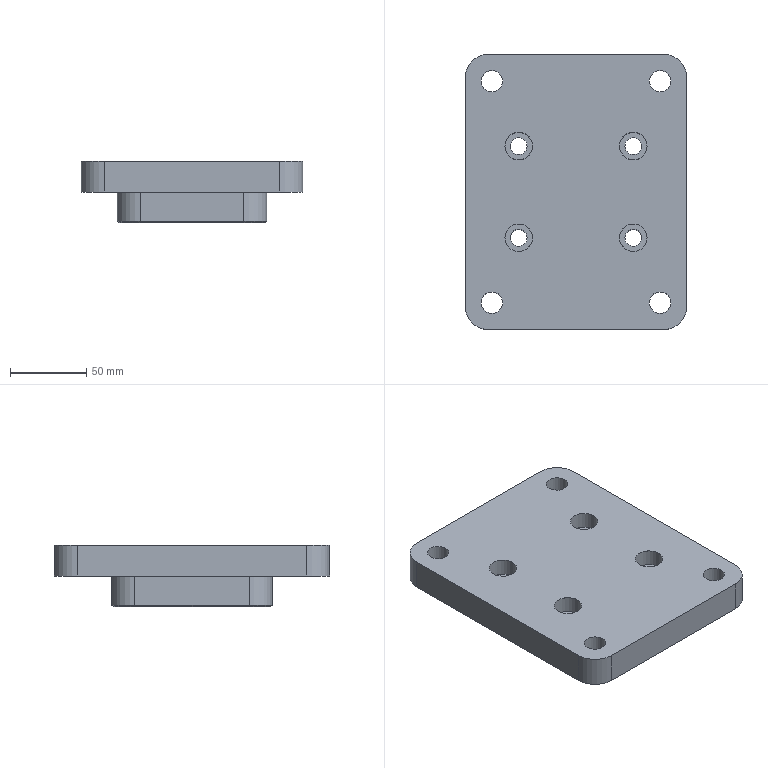Part | 1 solid | 47 faces | box 145 x 180 x 40 mm | volume 685350 mm3 | cylinder 20 | plane 19 | cone 8 | commonest cylinder face diameters 30 x8 11 x4 14 x4 18 x4
STEP:
#1=CARTESIAN_POINT('',(-32.,30.,-40.));
#2=VERTEX_POINT('',#1);
#3=CARTESIAN_POINT('',(-37.5,30.,-40.));
#4=DIRECTION('',(0.,0.,1.));
#5=DIRECTION('',(1.,0.,0.));
#6=AXIS2_PLACEMENT_3D('',#3,#4,#5);
#7=CIRCLE('',#6,5.5);
#8=EDGE_CURVE('',#2,#2,#7,.T.);
#9=ORIENTED_EDGE('',*,*,#8,.T.);
#10=EDGE_LOOP('',(#9));
#11=FACE_BOUND('',#10,.T.);
#12=CARTESIAN_POINT('',(43.,30.,-40.));
#13=VERTEX_POINT('',#12);
#14=CARTESIAN_POINT('',(37.5,30.,-40.));
#15=DIRECTION('',(0.,0.,1.));
#16=DIRECTION('',(1.,0.,0.));
#17=AXIS2_PLACEMENT_3D('',#14,#15,#16);
#18=CIRCLE('',#17,5.5);
#19=EDGE_CURVE('',#13,#13,#18,.T.);
#20=ORIENTED_EDGE('',*,*,#19,.T.);
#21=EDGE_LOOP('',(#20));
#22=FACE_BOUND('',#21,.T.);
#23=CARTESIAN_POINT('',(34.,51.5,-40.));
#24=VERTEX_POINT('',#23);
#25=CARTESIAN_POINT('',(48.,37.5,-40.));
#26=VERTEX_POINT('',#25);
#27=CARTESIAN_POINT('',(34.,37.5,-40.));
#28=DIRECTION('',(0.,0.,-1.));
#29=DIRECTION('',(-1.,0.,0.));
#30=AXIS2_PLACEMENT_3D('',#27,#28,#29);
#31=CIRCLE('',#30,14.);
#32=EDGE_CURVE('',#24,#26,#31,.T.);
#33=ORIENTED_EDGE('',*,*,#32,.T.);
#34=CARTESIAN_POINT('',(48.,-37.5,-40.));
#35=VERTEX_POINT('',#34);
#36=CARTESIAN_POINT('',(48.,-37.5,-40.));
#37=DIRECTION('',(0.,-1.,0.));
#38=VECTOR('',#37,1000.);
#39=LINE('',#36,#38);
#40=EDGE_CURVE('',#26,#35,#39,.T.);
#41=ORIENTED_EDGE('',*,*,#40,.T.);
#42=CARTESIAN_POINT('',(34.,-51.5,-40.));
#43=VERTEX_POINT('',#42);
#44=CARTESIAN_POINT('',(34.,-37.5,-40.));
#45=DIRECTION('',(0.,0.,-1.));
#46=DIRECTION('',(-1.,0.,0.));
#47=AXIS2_PLACEMENT_3D('',#44,#45,#46);
#48=CIRCLE('',#47,14.);
#49=EDGE_CURVE('',#35,#43,#48,.T.);
#50=ORIENTED_EDGE('',*,*,#49,.T.);
#51=CARTESIAN_POINT('',(-34.,-51.5,-40.));
#52=VERTEX_POINT('',#51);
#53=CARTESIAN_POINT('',(-34.,-51.5,-40.));
#54=DIRECTION('',(-1.,0.,0.));
#55=VECTOR('',#54,1000.);
#56=LINE('',#53,#55);
#57=EDGE_CURVE('',#43,#52,#56,.T.);
#58=ORIENTED_EDGE('',*,*,#57,.T.);
#59=CARTESIAN_POINT('',(-48.,-37.5,-40.));
#60=VERTEX_POINT('',#59);
#61=CARTESIAN_POINT('',(-34.,-37.5,-40.));
#62=DIRECTION('',(0.,0.,-1.));
#63=DIRECTION('',(-1.,0.,0.));
#64=AXIS2_PLACEMENT_3D('',#61,#62,#63);
#65=CIRCLE('',#64,14.);
#66=EDGE_CURVE('',#52,#60,#65,.T.);
#67=ORIENTED_EDGE('',*,*,#66,.T.);
#68=CARTESIAN_POINT('',(-48.,37.5,-40.));
#69=VERTEX_POINT('',#68);
#70=CARTESIAN_POINT('',(-48.,37.5,-40.));
#71=DIRECTION('',(0.,1.,0.));
#72=VECTOR('',#71,1000.);
#73=LINE('',#70,#72);
#74=EDGE_CURVE('',#60,#69,#73,.T.);
#75=ORIENTED_EDGE('',*,*,#74,.T.);
#76=CARTESIAN_POINT('',(-34.,51.5,-40.));
#77=VERTEX_POINT('',#76);
#78=CARTESIAN_POINT('',(-34.,37.5,-40.));
#79=DIRECTION('',(0.,0.,-1.));
#80=DIRECTION('',(-1.,0.,0.));
#81=AXIS2_PLACEMENT_3D('',#78,#79,#80);
#82=CIRCLE('',#81,14.);
#83=EDGE_CURVE('',#69,#77,#82,.T.);
#84=ORIENTED_EDGE('',*,*,#83,.T.);
#85=CARTESIAN_POINT('',(34.,51.5,-40.));
#86=DIRECTION('',(1.,0.,0.));
#87=VECTOR('',#86,1000.);
#88=LINE('',#85,#87);
#89=EDGE_CURVE('',#77,#24,#88,.T.);
#90=ORIENTED_EDGE('',*,*,#89,.T.);
#91=EDGE_LOOP('',(#33,#41,#50,#58,#67,#75,#84,#90));
#92=FACE_BOUND('',#91,.T.);
#93=CARTESIAN_POINT('',(43.,-30.,-40.));
#94=VERTEX_POINT('',#93);
#95=CARTESIAN_POINT('',(37.5,-30.,-40.));
#96=DIRECTION('',(0.,0.,1.));
#97=DIRECTION('',(1.,0.,0.));
#98=AXIS2_PLACEMENT_3D('',#95,#96,#97);
#99=CIRCLE('',#98,5.5);
#100=EDGE_CURVE('',#94,#94,#99,.T.);
#101=ORIENTED_EDGE('',*,*,#100,.T.);
#102=EDGE_LOOP('',(#101));
#103=FACE_BOUND('',#102,.T.);
#104=CARTESIAN_POINT('',(-32.,-30.,-40.));
#105=VERTEX_POINT('',#104);
#106=CARTESIAN_POINT('',(-37.5,-30.,-40.));
#107=DIRECTION('',(0.,0.,1.));
#108=DIRECTION('',(1.,0.,0.));
#109=AXIS2_PLACEMENT_3D('',#106,#107,#108);
#110=CIRCLE('',#109,5.5);
#111=EDGE_CURVE('',#105,#105,#110,.T.);
#112=ORIENTED_EDGE('',*,*,#111,.T.);
#113=EDGE_LOOP('',(#112));
#114=FACE_BOUND('',#113,.T.);
#115=CARTESIAN_POINT('',(34.,37.5,-40.));
#116=DIRECTION('',(0.,0.,-1.));
#117=DIRECTION('',(-1.,0.,0.));
#118=AXIS2_PLACEMENT_3D('',#115,#116,#117);
#119=PLANE('',#118);
#120=ADVANCED_FACE('',(#11,#22,#92,#103,#114),#119,.T.);
#121=CARTESIAN_POINT('',(49.,37.5,-20.));
#122=VERTEX_POINT('',#121);
#123=CARTESIAN_POINT('',(49.,37.5,-39.));
#124=VERTEX_POINT('',#123);
#125=CARTESIAN_POINT('',(49.,37.5,-20.));
#126=DIRECTION('',(0.,0.,-1.));
#127=VECTOR('',#126,1000.);
#128=LINE('',#125,#127);
#129=EDGE_CURVE('',#122,#124,#128,.T.);
#130=ORIENTED_EDGE('',*,*,#129,.T.);
#131=CARTESIAN_POINT('',(34.,52.5,-39.));
#132=VERTEX_POINT('',#131);
#133=CARTESIAN_POINT('',(34.,37.5,-39.));
#134=DIRECTION('',(0.,0.,-1.));
#135=DIRECTION('',(-1.,0.,0.));
#136=AXIS2_PLACEMENT_3D('',#133,#134,#135);
#137=CIRCLE('',#136,15.);
#138=EDGE_CURVE('',#124,#132,#137,.F.);
#139=ORIENTED_EDGE('',*,*,#138,.T.);
#140=CARTESIAN_POINT('',(34.,52.5,-20.));
#141=VERTEX_POINT('',#140);
#142=CARTESIAN_POINT('',(34.,52.5,-20.));
#143=DIRECTION('',(0.,0.,-1.));
#144=VECTOR('',#143,1000.);
#145=LINE('',#142,#144);
#146=EDGE_CURVE('',#141,#132,#145,.T.);
#147=ORIENTED_EDGE('',*,*,#146,.F.);
#148=CARTESIAN_POINT('',(34.,37.5,-20.));
#149=DIRECTION('',(0.,0.,1.));
#150=DIRECTION('',(-1.,0.,0.));
#151=AXIS2_PLACEMENT_3D('',#148,#149,#150);
#152=CIRCLE('',#151,15.);
#153=EDGE_CURVE('',#122,#141,#152,.T.);
#154=ORIENTED_EDGE('',*,*,#153,.F.);
#155=EDGE_LOOP('',(#130,#139,#147,#154));
#156=FACE_BOUND('',#155,.T.);
#157=CARTESIAN_POINT('',(34.,37.5,-20.));
#158=DIRECTION('',(0.,0.,-1.));
#159=DIRECTION('',(-1.,0.,0.));
#160=AXIS2_PLACEMENT_3D('',#157,#158,#159);
#161=CYLINDRICAL_SURFACE('',#160,15.);
#162=ADVANCED_FACE('',(#156),#161,.T.);
#163=ORIENTED_EDGE('',*,*,#146,.T.);
#164=CARTESIAN_POINT('',(-34.,52.5,-39.));
#165=VERTEX_POINT('',#164);
#166=CARTESIAN_POINT('',(-34.,52.5,-39.));
#167=DIRECTION('',(-1.,0.,0.));
#168=VECTOR('',#167,1000.);
#169=LINE('',#166,#168);
#170=EDGE_CURVE('',#132,#165,#169,.T.);
#171=ORIENTED_EDGE('',*,*,#170,.T.);
#172=CARTESIAN_POINT('',(-34.,52.5,-20.));
#173=VERTEX_POINT('',#172);
#174=CARTESIAN_POINT('',(-34.,52.5,-20.));
#175=DIRECTION('',(0.,0.,-1.));
#176=VECTOR('',#175,1000.);
#177=LINE('',#174,#176);
#178=EDGE_CURVE('',#173,#165,#177,.T.);
#179=ORIENTED_EDGE('',*,*,#178,.F.);
#180=CARTESIAN_POINT('',(-34.,52.5,-20.));
#181=DIRECTION('',(-1.,0.,0.));
#182=VECTOR('',#181,1000.);
#183=LINE('',#180,#182);
#184=EDGE_CURVE('',#141,#173,#183,.T.);
#185=ORIENTED_EDGE('',*,*,#184,.F.);
#186=EDGE_LOOP('',(#163,#171,#179,#185));
#187=FACE_BOUND('',#186,.T.);
#188=CARTESIAN_POINT('',(-34.,52.5,-20.));
#189=DIRECTION('',(0.,-1.,0.));
#190=DIRECTION('',(0.,0.,-1.));
#191=AXIS2_PLACEMENT_3D('',#188,#189,#190);
#192=PLANE('',#191);
#193=ADVANCED_FACE('',(#187),#192,.F.);
#194=ORIENTED_EDGE('',*,*,#178,.T.);
#195=CARTESIAN_POINT('',(-49.,37.5,-39.));
#196=VERTEX_POINT('',#195);
#197=CARTESIAN_POINT('',(-34.,37.5,-39.));
#198=DIRECTION('',(0.,0.,-1.));
#199=DIRECTION('',(-1.,0.,0.));
#200=AXIS2_PLACEMENT_3D('',#197,#198,#199);
#201=CIRCLE('',#200,15.);
#202=EDGE_CURVE('',#165,#196,#201,.F.);
#203=ORIENTED_EDGE('',*,*,#202,.T.);
#204=CARTESIAN_POINT('',(-49.,37.5,-20.));
#205=VERTEX_POINT('',#204);
#206=CARTESIAN_POINT('',(-49.,37.5,-20.));
#207=DIRECTION('',(0.,0.,-1.));
#208=VECTOR('',#207,1000.);
#209=LINE('',#206,#208);
#210=EDGE_CURVE('',#205,#196,#209,.T.);
#211=ORIENTED_EDGE('',*,*,#210,.F.);
#212=CARTESIAN_POINT('',(-34.,37.5,-20.));
#213=DIRECTION('',(0.,0.,1.));
#214=DIRECTION('',(1.,0.,0.));
#215=AXIS2_PLACEMENT_3D('',#212,#213,#214);
#216=CIRCLE('',#215,15.);
#217=EDGE_CURVE('',#173,#205,#216,.T.);
#218=ORIENTED_EDGE('',*,*,#217,.F.);
#219=EDGE_LOOP('',(#194,#203,#211,#218));
#220=FACE_BOUND('',#219,.T.);
#221=CARTESIAN_POINT('',(-34.,37.5,-20.));
#222=DIRECTION('',(0.,0.,-1.));
#223=DIRECTION('',(-1.,0.,0.));
#224=AXIS2_PLACEMENT_3D('',#221,#222,#223);
#225=CYLINDRICAL_SURFACE('',#224,15.);
#226=ADVANCED_FACE('',(#220),#225,.T.);
#227=ORIENTED_EDGE('',*,*,#210,.T.);
#228=CARTESIAN_POINT('',(-49.,-37.5,-39.));
#229=VERTEX_POINT('',#228);
#230=CARTESIAN_POINT('',(-49.,-37.5,-39.));
#231=DIRECTION('',(0.,-1.,0.));
#232=VECTOR('',#231,1000.);
#233=LINE('',#230,#232);
#234=EDGE_CURVE('',#196,#229,#233,.T.);
#235=ORIENTED_EDGE('',*,*,#234,.T.);
#236=CARTESIAN_POINT('',(-49.,-37.5,-20.));
#237=VERTEX_POINT('',#236);
#238=CARTESIAN_POINT('',(-49.,-37.5,-20.));
#239=DIRECTION('',(0.,0.,-1.));
#240=VECTOR('',#239,1000.);
#241=LINE('',#238,#240);
#242=EDGE_CURVE('',#237,#229,#241,.T.);
#243=ORIENTED_EDGE('',*,*,#242,.F.);
#244=CARTESIAN_POINT('',(-49.,37.5,-20.));
#245=DIRECTION('',(0.,-1.,0.));
#246=VECTOR('',#245,1000.);
#247=LINE('',#244,#246);
#248=EDGE_CURVE('',#205,#237,#247,.T.);
#249=ORIENTED_EDGE('',*,*,#248,.F.);
#250=EDGE_LOOP('',(#227,#235,#243,#249));
#251=FACE_BOUND('',#250,.T.);
#252=CARTESIAN_POINT('',(-49.,37.5,-20.));
#253=DIRECTION('',(1.,0.,0.));
#254=DIRECTION('',(0.,1.,0.));
#255=AXIS2_PLACEMENT_3D('',#252,#253,#254);
#256=PLANE('',#255);
#257=ADVANCED_FACE('',(#251),#256,.F.);
#258=ORIENTED_EDGE('',*,*,#242,.T.);
#259=CARTESIAN_POINT('',(-34.,-52.5,-39.));
#260=VERTEX_POINT('',#259);
#261=CARTESIAN_POINT('',(-34.,-37.5,-39.));
#262=DIRECTION('',(0.,0.,-1.));
#263=DIRECTION('',(-1.,0.,0.));
#264=AXIS2_PLACEMENT_3D('',#261,#262,#263);
#265=CIRCLE('',#264,15.);
#266=EDGE_CURVE('',#229,#260,#265,.F.);
#267=ORIENTED_EDGE('',*,*,#266,.T.);
#268=CARTESIAN_POINT('',(-34.,-52.5,-20.));
#269=VERTEX_POINT('',#268);
#270=CARTESIAN_POINT('',(-34.,-52.5,-20.));
#271=DIRECTION('',(0.,0.,-1.));
#272=VECTOR('',#271,1000.);
#273=LINE('',#270,#272);
#274=EDGE_CURVE('',#269,#260,#273,.T.);
#275=ORIENTED_EDGE('',*,*,#274,.F.);
#276=CARTESIAN_POINT('',(-34.,-37.5,-20.));
#277=DIRECTION('',(0.,0.,1.));
#278=DIRECTION('',(1.,0.,0.));
#279=AXIS2_PLACEMENT_3D('',#276,#277,#278);
#280=CIRCLE('',#279,15.);
#281=EDGE_CURVE('',#237,#269,#280,.T.);
#282=ORIENTED_EDGE('',*,*,#281,.F.);
#283=EDGE_LOOP('',(#258,#267,#275,#282));
#284=FACE_BOUND('',#283,.T.);
#285=CARTESIAN_POINT('',(-34.,-37.5,-20.));
#286=DIRECTION('',(0.,0.,-1.));
#287=DIRECTION('',(-1.,0.,0.));
#288=AXIS2_PLACEMENT_3D('',#285,#286,#287);
#289=CYLINDRICAL_SURFACE('',#288,15.);
#290=ADVANCED_FACE('',(#284),#289,.T.);
#291=ORIENTED_EDGE('',*,*,#274,.T.);
#292=CARTESIAN_POINT('',(34.,-52.5,-39.));
#293=VERTEX_POINT('',#292);
#294=CARTESIAN_POINT('',(34.,-52.5,-39.));
#295=DIRECTION('',(1.,0.,0.));
#296=VECTOR('',#295,1000.);
#297=LINE('',#294,#296);
#298=EDGE_CURVE('',#260,#293,#297,.T.);
#299=ORIENTED_EDGE('',*,*,#298,.T.);
#300=CARTESIAN_POINT('',(34.,-52.5,-20.));
#301=VERTEX_POINT('',#300);
#302=CARTESIAN_POINT('',(34.,-52.5,-20.));
#303=DIRECTION('',(0.,0.,-1.));
#304=VECTOR('',#303,1000.);
#305=LINE('',#302,#304);
#306=EDGE_CURVE('',#301,#293,#305,.T.);
#307=ORIENTED_EDGE('',*,*,#306,.F.);
#308=CARTESIAN_POINT('',(-34.,-52.5,-20.));
#309=DIRECTION('',(1.,0.,0.));
#310=VECTOR('',#309,1000.);
#311=LINE('',#308,#310);
#312=EDGE_CURVE('',#269,#301,#311,.T.);
#313=ORIENTED_EDGE('',*,*,#312,.F.);
#314=EDGE_LOOP('',(#291,#299,#307,#313));
#315=FACE_BOUND('',#314,.T.);
#316=CARTESIAN_POINT('',(-34.,-52.5,-20.));
#317=DIRECTION('',(0.,1.,0.));
#318=DIRECTION('',(0.,0.,1.));
#319=AXIS2_PLACEMENT_3D('',#316,#317,#318);
#320=PLANE('',#319);
#321=ADVANCED_FACE('',(#315),#320,.F.);
#322=ORIENTED_EDGE('',*,*,#306,.T.);
#323=CARTESIAN_POINT('',(49.,-37.5,-39.));
#324=VERTEX_POINT('',#323);
#325=CARTESIAN_POINT('',(34.,-37.5,-39.));
#326=DIRECTION('',(0.,0.,-1.));
#327=DIRECTION('',(-1.,0.,0.));
#328=AXIS2_PLACEMENT_3D('',#325,#326,#327);
#329=CIRCLE('',#328,15.);
#330=EDGE_CURVE('',#293,#324,#329,.F.);
#331=ORIENTED_EDGE('',*,*,#330,.T.);
#332=CARTESIAN_POINT('',(49.,-37.5,-20.));
#333=VERTEX_POINT('',#332);
#334=CARTESIAN_POINT('',(49.,-37.5,-20.));
#335=DIRECTION('',(0.,0.,-1.));
#336=VECTOR('',#335,1000.);
#337=LINE('',#334,#336);
#338=EDGE_CURVE('',#333,#324,#337,.T.);
#339=ORIENTED_EDGE('',*,*,#338,.F.);
#340=CARTESIAN_POINT('',(34.,-37.5,-20.));
#341=DIRECTION('',(0.,0.,1.));
#342=DIRECTION('',(1.,0.,0.));
#343=AXIS2_PLACEMENT_3D('',#340,#341,#342);
#344=CIRCLE('',#343,15.);
#345=EDGE_CURVE('',#301,#333,#344,.T.);
#346=ORIENTED_EDGE('',*,*,#345,.F.);
#347=EDGE_LOOP('',(#322,#331,#339,#346));
#348=FACE_BOUND('',#347,.T.);
#349=CARTESIAN_POINT('',(34.,-37.5,-20.));
#350=DIRECTION('',(0.,0.,-1.));
#351=DIRECTION('',(-1.,0.,0.));
#352=AXIS2_PLACEMENT_3D('',#349,#350,#351);
#353=CYLINDRICAL_SURFACE('',#352,15.);
#354=ADVANCED_FACE('',(#348),#353,.T.);
#355=ORIENTED_EDGE('',*,*,#338,.T.);
#356=CARTESIAN_POINT('',(49.,37.5,-39.));
#357=DIRECTION('',(0.,1.,0.));
#358=VECTOR('',#357,1000.);
#359=LINE('',#356,#358);
#360=EDGE_CURVE('',#324,#124,#359,.T.);
#361=ORIENTED_EDGE('',*,*,#360,.T.);
#362=ORIENTED_EDGE('',*,*,#129,.F.);
#363=CARTESIAN_POINT('',(49.,37.5,-20.));
#364=DIRECTION('',(0.,1.,0.));
#365=VECTOR('',#364,1000.);
#366=LINE('',#363,#365);
#367=EDGE_CURVE('',#333,#122,#366,.T.);
#368=ORIENTED_EDGE('',*,*,#367,.F.);
#369=EDGE_LOOP('',(#355,#361,#362,#368));
#370=FACE_BOUND('',#369,.T.);
#371=CARTESIAN_POINT('',(49.,37.5,-20.));
#372=DIRECTION('',(-1.,0.,0.));
#373=DIRECTION('',(0.,-1.,0.));
#374=AXIS2_PLACEMENT_3D('',#371,#372,#373);
#375=PLANE('',#374);
#376=ADVANCED_FACE('',(#370),#375,.F.);
#377=CARTESIAN_POINT('',(-72.5,75.,-20.));
#378=VERTEX_POINT('',#377);
#379=CARTESIAN_POINT('',(-72.5,-75.,-20.));
#380=VERTEX_POINT('',#379);
#381=CARTESIAN_POINT('',(-72.5,90.,-20.));
#382=DIRECTION('',(0.,-1.,0.));
#383=VECTOR('',#382,1000.);
#384=LINE('',#381,#383);
#385=EDGE_CURVE('',#378,#380,#384,.T.);
#386=ORIENTED_EDGE('',*,*,#385,.T.);
#387=CARTESIAN_POINT('',(-72.5,-75.,0.));
#388=VERTEX_POINT('',#387);
#389=CARTESIAN_POINT('',(-72.5,-75.,0.));
#390=DIRECTION('',(0.,0.,-1.));
#391=VECTOR('',#390,1000.);
#392=LINE('',#389,#391);
#393=EDGE_CURVE('',#380,#388,#392,.F.);
#394=ORIENTED_EDGE('',*,*,#393,.T.);
#395=CARTESIAN_POINT('',(-72.5,75.,0.));
#396=VERTEX_POINT('',#395);
#397=CARTESIAN_POINT('',(-72.5,90.,0.));
#398=DIRECTION('',(0.,-1.,0.));
#399=VECTOR('',#398,1000.);
#400=LINE('',#397,#399);
#401=EDGE_CURVE('',#396,#388,#400,.T.);
#402=ORIENTED_EDGE('',*,*,#401,.F.);
#403=CARTESIAN_POINT('',(-72.5,75.,0.));
#404=DIRECTION('',(0.,0.,-1.));
#405=VECTOR('',#404,1000.);
#406=LINE('',#403,#405);
#407=EDGE_CURVE('',#396,#378,#406,.T.);
#408=ORIENTED_EDGE('',*,*,#407,.T.);
#409=EDGE_LOOP('',(#386,#394,#402,#408));
#410=FACE_BOUND('',#409,.T.);
#411=CARTESIAN_POINT('',(-72.5,90.,0.));
#412=DIRECTION('',(1.,0.,0.));
#413=DIRECTION('',(0.,1.,0.));
#414=AXIS2_PLACEMENT_3D('',#411,#412,#413);
#415=PLANE('',#414);
#416=ADVANCED_FACE('',(#410),#415,.F.);
#417=CARTESIAN_POINT('',(-57.5,-90.,-20.));
#418=VERTEX_POINT('',#417);
#419=CARTESIAN_POINT('',(57.5,-90.,-20.));
#420=VERTEX_POINT('',#419);
#421=CARTESIAN_POINT('',(72.5,-90.,-20.));
#422=DIRECTION('',(1.,0.,0.));
#423=VECTOR('',#422,1000.);
#424=LINE('',#421,#423);
#425=EDGE_CURVE('',#418,#420,#424,.T.);
#426=ORIENTED_EDGE('',*,*,#425,.T.);
#427=CARTESIAN_POINT('',(57.5,-90.,0.));
#428=VERTEX_POINT('',#427);
#429=CARTESIAN_POINT('',(57.5,-90.,0.));
#430=DIRECTION('',(0.,0.,-1.));
#431=VECTOR('',#430,1000.);
#432=LINE('',#429,#431);
#433=EDGE_CURVE('',#420,#428,#432,.F.);
#434=ORIENTED_EDGE('',*,*,#433,.T.);
#435=CARTESIAN_POINT('',(-57.5,-90.,0.));
#436=VERTEX_POINT('',#435);
#437=CARTESIAN_POINT('',(72.5,-90.,0.));
#438=DIRECTION('',(1.,0.,0.));
#439=VECTOR('',#438,1000.);
#440=LINE('',#437,#439);
#441=EDGE_CURVE('',#436,#428,#440,.T.);
#442=ORIENTED_EDGE('',*,*,#441,.F.);
#443=CARTESIAN_POINT('',(-57.5,-90.,0.));
#444=DIRECTION('',(0.,0.,-1.));
#445=VECTOR('',#444,1000.);
#446=LINE('',#443,#445);
#447=EDGE_CURVE('',#436,#418,#446,.T.);
#448=ORIENTED_EDGE('',*,*,#447,.T.);
#449=EDGE_LOOP('',(#426,#434,#442,#448));
#450=FACE_BOUND('',#449,.T.);
#451=CARTESIAN_POINT('',(72.5,-90.,0.));
#452=DIRECTION('',(0.,1.,0.));
#453=DIRECTION('',(-1.,0.,0.));
#454=AXIS2_PLACEMENT_3D('',#451,#452,#453);
#455=PLANE('',#454);
#456=ADVANCED_FACE('',(#450),#455,.F.);
#457=CARTESIAN_POINT('',(72.5,-75.,0.));
#458=VERTEX_POINT('',#457);
#459=CARTESIAN_POINT('',(72.5,75.,0.));
#460=VERTEX_POINT('',#459);
#461=CARTESIAN_POINT('',(72.5,90.,0.));
#462=DIRECTION('',(0.,1.,0.));
#463=VECTOR('',#462,1000.);
#464=LINE('',#461,#463);
#465=EDGE_CURVE('',#458,#460,#464,.T.);
#466=ORIENTED_EDGE('',*,*,#465,.F.);
#467=CARTESIAN_POINT('',(72.5,-75.,-20.));
#468=VERTEX_POINT('',#467);
#469=CARTESIAN_POINT('',(72.5,-75.,0.));
#470=DIRECTION('',(0.,0.,-1.));
#471=VECTOR('',#470,1000.);
#472=LINE('',#469,#471);
#473=EDGE_CURVE('',#458,#468,#472,.T.);
#474=ORIENTED_EDGE('',*,*,#473,.T.);
#475=CARTESIAN_POINT('',(72.5,75.,-20.));
#476=VERTEX_POINT('',#475);
#477=CARTESIAN_POINT('',(72.5,90.,-20.));
#478=DIRECTION('',(0.,1.,0.));
#479=VECTOR('',#478,1000.);
#480=LINE('',#477,#479);
#481=EDGE_CURVE('',#468,#476,#480,.T.);
#482=ORIENTED_EDGE('',*,*,#481,.T.);
#483=CARTESIAN_POINT('',(72.5,75.,0.));
#484=DIRECTION('',(0.,0.,-1.));
#485=VECTOR('',#484,1000.);
#486=LINE('',#483,#485);
#487=EDGE_CURVE('',#476,#460,#486,.F.);
#488=ORIENTED_EDGE('',*,*,#487,.T.);
#489=EDGE_LOOP('',(#466,#474,#482,#488));
#490=FACE_BOUND('',#489,.T.);
#491=CARTESIAN_POINT('',(72.5,90.,0.));
#492=DIRECTION('',(-1.,0.,0.));
#493=DIRECTION('',(0.,-1.,0.));
#494=AXIS2_PLACEMENT_3D('',#491,#492,#493);
#495=PLANE('',#494);
#496=ADVANCED_FACE('',(#490),#495,.F.);
#497=CARTESIAN_POINT('',(57.5,90.,0.));
#498=VERTEX_POINT('',#497);
#499=CARTESIAN_POINT('',(-57.5,90.,0.));
#500=VERTEX_POINT('',#499);
#501=CARTESIAN_POINT('',(72.5,90.,0.));
#502=DIRECTION('',(-1.,0.,0.));
#503=VECTOR('',#502,1000.);
#504=LINE('',#501,#503);
#505=EDGE_CURVE('',#498,#500,#504,.T.);
#506=ORIENTED_EDGE('',*,*,#505,.F.);
#507=CARTESIAN_POINT('',(57.5,90.,-20.));
#508=VERTEX_POINT('',#507);
#509=CARTESIAN_POINT('',(57.5,90.,0.));
#510=DIRECTION('',(0.,0.,-1.));
#511=VECTOR('',#510,1000.);
#512=LINE('',#509,#511);
#513=EDGE_CURVE('',#498,#508,#512,.T.);
#514=ORIENTED_EDGE('',*,*,#513,.T.);
#515=CARTESIAN_POINT('',(-57.5,90.,-20.));
#516=VERTEX_POINT('',#515);
#517=CARTESIAN_POINT('',(72.5,90.,-20.));
#518=DIRECTION('',(-1.,0.,0.));
#519=VECTOR('',#518,1000.);
#520=LINE('',#517,#519);
#521=EDGE_CURVE('',#508,#516,#520,.T.);
#522=ORIENTED_EDGE('',*,*,#521,.T.);
#523=CARTESIAN_POINT('',(-57.5,90.,0.));
#524=DIRECTION('',(0.,0.,-1.));
#525=VECTOR('',#524,1000.);
#526=LINE('',#523,#525);
#527=EDGE_CURVE('',#516,#500,#526,.F.);
#528=ORIENTED_EDGE('',*,*,#527,.T.);
#529=EDGE_LOOP('',(#506,#514,#522,#528));
#530=FACE_BOUND('',#529,.T.);
#531=CARTESIAN_POINT('',(72.5,90.,0.));
#532=DIRECTION('',(0.,-1.,0.));
#533=DIRECTION('',(1.,0.,0.));
#534=AXIS2_PLACEMENT_3D('',#531,#532,#533);
#535=PLANE('',#534);
#536=ADVANCED_FACE('',(#530),#535,.F.);
#537=CARTESIAN_POINT('',(-28.475,30.,0.));
#538=VERTEX_POINT('',#537);
#539=CARTESIAN_POINT('',(-37.5,30.,0.));
#540=DIRECTION('',(0.,0.,1.));
#541=DIRECTION('',(1.,0.,0.));
#542=AXIS2_PLACEMENT_3D('',#539,#540,#541);
#543=CIRCLE('',#542,9.025);
#544=EDGE_CURVE('',#538,#538,#543,.T.);
#545=ORIENTED_EDGE('',*,*,#544,.F.);
#546=EDGE_LOOP('',(#545));
#547=FACE_BOUND('',#546,.T.);
#548=CARTESIAN_POINT('',(46.525,30.,0.));
#549=VERTEX_POINT('',#548);
#550=CARTESIAN_POINT('',(37.5,30.,0.));
#551=DIRECTION('',(0.,0.,1.));
#552=DIRECTION('',(1.,0.,0.));
#553=AXIS2_PLACEMENT_3D('',#550,#551,#552);
#554=CIRCLE('',#553,9.025);
#555=EDGE_CURVE('',#549,#549,#554,.T.);
#556=ORIENTED_EDGE('',*,*,#555,.F.);
#557=EDGE_LOOP('',(#556));
#558=FACE_BOUND('',#557,.T.);
#559=CARTESIAN_POINT('',(-28.475,-30.,0.));
#560=VERTEX_POINT('',#559);
#561=CARTESIAN_POINT('',(-37.5,-30.,0.));
#562=DIRECTION('',(0.,0.,1.));
#563=DIRECTION('',(1.,0.,0.));
#564=AXIS2_PLACEMENT_3D('',#561,#562,#563);
#565=CIRCLE('',#564,9.025);
#566=EDGE_CURVE('',#560,#560,#565,.T.);
#567=ORIENTED_EDGE('',*,*,#566,.F.);
#568=EDGE_LOOP('',(#567));
#569=FACE_BOUND('',#568,.T.);
#570=CARTESIAN_POINT('',(46.525,-30.,0.));
#571=VERTEX_POINT('',#570);
#572=CARTESIAN_POINT('',(37.5,-30.,0.));
#573=DIRECTION('',(0.,0.,1.));
#574=DIRECTION('',(1.,0.,0.));
#575=AXIS2_PLACEMENT_3D('',#572,#573,#574);
#576=CIRCLE('',#575,9.025);
#577=EDGE_CURVE('',#571,#571,#576,.T.);
#578=ORIENTED_EDGE('',*,*,#577,.F.);
#579=EDGE_LOOP('',(#578));
#580=FACE_BOUND('',#579,.T.);
#581=CARTESIAN_POINT('',(-48.,72.5,0.));
#582=VERTEX_POINT('',#581);
#583=CARTESIAN_POINT('',(-55.,72.5,0.));
#584=DIRECTION('',(0.,0.,-1.));
#585=DIRECTION('',(1.,0.,0.));
#586=AXIS2_PLACEMENT_3D('',#583,#584,#585);
#587=CIRCLE('',#586,7.);
#588=EDGE_CURVE('',#582,#582,#587,.T.);
#589=ORIENTED_EDGE('',*,*,#588,.T.);
#590=EDGE_LOOP('',(#589));
#591=FACE_BOUND('',#590,.T.);
#592=CARTESIAN_POINT('',(48.,72.5,0.));
#593=VERTEX_POINT('',#592);
#594=CARTESIAN_POINT('',(55.,72.5,0.));
#595=DIRECTION('',(0.,0.,-1.));
#596=DIRECTION('',(-1.,0.,0.));
#597=AXIS2_PLACEMENT_3D('',#594,#595,#596);
#598=CIRCLE('',#597,7.);
#599=EDGE_CURVE('',#593,#593,#598,.T.);
#600=ORIENTED_EDGE('',*,*,#599,.T.);
#601=EDGE_LOOP('',(#600));
#602=FACE_BOUND('',#601,.T.);
#603=CARTESIAN_POINT('',(62.,-72.5,0.));
#604=VERTEX_POINT('',#603);
#605=CARTESIAN_POINT('',(55.,-72.5,0.));
#606=DIRECTION('',(0.,0.,-1.));
#607=DIRECTION('',(1.,0.,0.));
#608=AXIS2_PLACEMENT_3D('',#605,#606,#607);
#609=CIRCLE('',#608,7.);
#610=EDGE_CURVE('',#604,#604,#609,.T.);
#611=ORIENTED_EDGE('',*,*,#610,.T.);
#612=EDGE_LOOP('',(#611));
#613=FACE_BOUND('',#612,.T.);
#614=CARTESIAN_POINT('',(-62.,-72.5,0.));
#615=VERTEX_POINT('',#614);
#616=CARTESIAN_POINT('',(-55.,-72.5,0.));
#617=DIRECTION('',(0.,0.,-1.));
#618=DIRECTION('',(-1.,0.,0.));
#619=AXIS2_PLACEMENT_3D('',#616,#617,#618);
#620=CIRCLE('',#619,7.);
#621=EDGE_CURVE('',#615,#615,#620,.T.);
#622=ORIENTED_EDGE('',*,*,#621,.T.);
#623=EDGE_LOOP('',(#622));
#624=FACE_BOUND('',#623,.T.);
#625=ORIENTED_EDGE('',*,*,#441,.T.);
#626=CARTESIAN_POINT('',(57.5,-75.,0.));
#627=DIRECTION('',(0.,0.,-1.));
#628=DIRECTION('',(-1.,0.,0.));
#629=AXIS2_PLACEMENT_3D('',#626,#627,#628);
#630=CIRCLE('',#629,15.);
#631=EDGE_CURVE('',#428,#458,#630,.F.);
#632=ORIENTED_EDGE('',*,*,#631,.T.);
#633=ORIENTED_EDGE('',*,*,#465,.T.);
#634=CARTESIAN_POINT('',(57.5,75.,0.));
#635=DIRECTION('',(0.,0.,-1.));
#636=DIRECTION('',(-1.,0.,0.));
#637=AXIS2_PLACEMENT_3D('',#634,#635,#636);
#638=CIRCLE('',#637,15.);
#639=EDGE_CURVE('',#460,#498,#638,.F.);
#640=ORIENTED_EDGE('',*,*,#639,.T.);
#641=ORIENTED_EDGE('',*,*,#505,.T.);
#642=CARTESIAN_POINT('',(-57.5,75.,0.));
#643=DIRECTION('',(0.,0.,-1.));
#644=DIRECTION('',(-1.,0.,0.));
#645=AXIS2_PLACEMENT_3D('',#642,#643,#644);
#646=CIRCLE('',#645,15.);
#647=EDGE_CURVE('',#500,#396,#646,.F.);
#648=ORIENTED_EDGE('',*,*,#647,.T.);
#649=ORIENTED_EDGE('',*,*,#401,.T.);
#650=CARTESIAN_POINT('',(-57.5,-75.,0.));
#651=DIRECTION('',(0.,0.,-1.));
#652=DIRECTION('',(-1.,0.,0.));
#653=AXIS2_PLACEMENT_3D('',#650,#651,#652);
#654=CIRCLE('',#653,15.);
#655=EDGE_CURVE('',#388,#436,#654,.F.);
#656=ORIENTED_EDGE('',*,*,#655,.T.);
#657=EDGE_LOOP('',(#625,#632,#633,#640,#641,#648,#649,#656));
#658=FACE_BOUND('',#657,.T.);
#659=CARTESIAN_POINT('',(0.,0.,0.));
#660=DIRECTION('',(0.,0.,-1.));
#661=DIRECTION('',(-1.,0.,0.));
#662=AXIS2_PLACEMENT_3D('',#659,#660,#661);
#663=PLANE('',#662);
#664=ADVANCED_FACE('',(#547,#558,#569,#580,#591,#602,#613,#624,#658),#663,.F.);
#665=CARTESIAN_POINT('',(-48.,72.5,-20.));
#666=VERTEX_POINT('',#665);
#667=CARTESIAN_POINT('',(-55.,72.5,-20.));
#668=DIRECTION('',(0.,0.,-1.));
#669=DIRECTION('',(1.,0.,0.));
#670=AXIS2_PLACEMENT_3D('',#667,#668,#669);
#671=CIRCLE('',#670,7.);
#672=EDGE_CURVE('',#666,#666,#671,.T.);
#673=ORIENTED_EDGE('',*,*,#672,.F.);
#674=EDGE_LOOP('',(#673));
#675=FACE_BOUND('',#674,.T.);
#676=CARTESIAN_POINT('',(48.,72.5,-20.));
#677=VERTEX_POINT('',#676);
#678=CARTESIAN_POINT('',(55.,72.5,-20.));
#679=DIRECTION('',(0.,0.,-1.));
#680=DIRECTION('',(-1.,0.,0.));
#681=AXIS2_PLACEMENT_3D('',#678,#679,#680);
#682=CIRCLE('',#681,7.);
#683=EDGE_CURVE('',#677,#677,#682,.T.);
#684=ORIENTED_EDGE('',*,*,#683,.F.);
#685=EDGE_LOOP('',(#684));
#686=FACE_BOUND('',#685,.T.);
#687=CARTESIAN_POINT('',(62.,-72.5,-20.));
#688=VERTEX_POINT('',#687);
#689=CARTESIAN_POINT('',(55.,-72.5,-20.));
#690=DIRECTION('',(0.,0.,-1.));
#691=DIRECTION('',(1.,0.,0.));
#692=AXIS2_PLACEMENT_3D('',#689,#690,#691);
#693=CIRCLE('',#692,7.);
#694=EDGE_CURVE('',#688,#688,#693,.T.);
#695=ORIENTED_EDGE('',*,*,#694,.F.);
#696=EDGE_LOOP('',(#695));
#697=FACE_BOUND('',#696,.T.);
#698=CARTESIAN_POINT('',(-62.,-72.5,-20.));
#699=VERTEX_POINT('',#698);
#700=CARTESIAN_POINT('',(-55.,-72.5,-20.));
#701=DIRECTION('',(0.,0.,-1.));
#702=DIRECTION('',(-1.,0.,0.));
#703=AXIS2_PLACEMENT_3D('',#700,#701,#702);
#704=CIRCLE('',#703,7.);
#705=EDGE_CURVE('',#699,#699,#704,.T.);
#706=ORIENTED_EDGE('',*,*,#705,.F.);
#707=EDGE_LOOP('',(#706));
#708=FACE_BOUND('',#707,.T.);
#709=ORIENTED_EDGE('',*,*,#367,.T.);
#710=ORIENTED_EDGE('',*,*,#153,.T.);
#711=ORIENTED_EDGE('',*,*,#184,.T.);
#712=ORIENTED_EDGE('',*,*,#217,.T.);
#713=ORIENTED_EDGE('',*,*,#248,.T.);
#714=ORIENTED_EDGE('',*,*,#281,.T.);
#715=ORIENTED_EDGE('',*,*,#312,.T.);
#716=ORIENTED_EDGE('',*,*,#345,.T.);
#717=EDGE_LOOP('',(#709,#710,#711,#712,#713,#714,#715,#716));
#718=FACE_BOUND('',#717,.T.);
#719=ORIENTED_EDGE('',*,*,#481,.F.);
#720=CARTESIAN_POINT('',(57.5,-75.,-20.));
#721=DIRECTION('',(0.,0.,-1.));
#722=DIRECTION('',(-1.,0.,0.));
#723=AXIS2_PLACEMENT_3D('',#720,#721,#722);
#724=CIRCLE('',#723,15.);
#725=EDGE_CURVE('',#468,#420,#724,.T.);
#726=ORIENTED_EDGE('',*,*,#725,.T.);
#727=ORIENTED_EDGE('',*,*,#425,.F.);
#728=CARTESIAN_POINT('',(-57.5,-75.,-20.));
#729=DIRECTION('',(0.,0.,-1.));
#730=DIRECTION('',(-1.,0.,0.));
#731=AXIS2_PLACEMENT_3D('',#728,#729,#730);
#732=CIRCLE('',#731,15.);
#733=EDGE_CURVE('',#418,#380,#732,.T.);
#734=ORIENTED_EDGE('',*,*,#733,.T.);
#735=ORIENTED_EDGE('',*,*,#385,.F.);
#736=CARTESIAN_POINT('',(-57.5,75.,-20.));
#737=DIRECTION('',(0.,0.,-1.));
#738=DIRECTION('',(-1.,0.,0.));
#739=AXIS2_PLACEMENT_3D('',#736,#737,#738);
#740=CIRCLE('',#739,15.);
#741=EDGE_CURVE('',#378,#516,#740,.T.);
#742=ORIENTED_EDGE('',*,*,#741,.T.);
#743=ORIENTED_EDGE('',*,*,#521,.F.);
#744=CARTESIAN_POINT('',(57.5,75.,-20.));
#745=DIRECTION('',(0.,0.,-1.));
#746=DIRECTION('',(-1.,0.,0.));
#747=AXIS2_PLACEMENT_3D('',#744,#745,#746);
#748=CIRCLE('',#747,15.);
#749=EDGE_CURVE('',#508,#476,#748,.T.);
#750=ORIENTED_EDGE('',*,*,#749,.T.);
#751=EDGE_LOOP('',(#719,#726,#727,#734,#735,#742,#743,#750));
#752=FACE_BOUND('',#751,.T.);
#753=CARTESIAN_POINT('',(0.,0.,-20.));
#754=DIRECTION('',(0.,0.,-1.));
#755=DIRECTION('',(-1.,0.,0.));
#756=AXIS2_PLACEMENT_3D('',#753,#754,#755);
#757=PLANE('',#756);
#758=ADVANCED_FACE('',(#675,#686,#697,#708,#718,#752),#757,.T.);
#759=ORIENTED_EDGE('',*,*,#631,.F.);
#760=ORIENTED_EDGE('',*,*,#433,.F.);
#761=ORIENTED_EDGE('',*,*,#725,.F.);
#762=ORIENTED_EDGE('',*,*,#473,.F.);
#763=EDGE_LOOP('',(#759,#760,#761,#762));
#764=FACE_BOUND('',#763,.T.);
#765=CARTESIAN_POINT('',(57.5,-75.,0.));
#766=DIRECTION('',(0.,0.,-1.));
#767=DIRECTION('',(-1.,0.,0.));
#768=AXIS2_PLACEMENT_3D('',#765,#766,#767);
#769=CYLINDRICAL_SURFACE('',#768,15.);
#770=ADVANCED_FACE('',(#764),#769,.T.);
#771=ORIENTED_EDGE('',*,*,#655,.F.);
#772=ORIENTED_EDGE('',*,*,#393,.F.);
#773=ORIENTED_EDGE('',*,*,#733,.F.);
#774=ORIENTED_EDGE('',*,*,#447,.F.);
#775=EDGE_LOOP('',(#771,#772,#773,#774));
#776=FACE_BOUND('',#775,.T.);
#777=CARTESIAN_POINT('',(-57.5,-75.,0.));
#778=DIRECTION('',(0.,0.,-1.));
#779=DIRECTION('',(-1.,0.,0.));
#780=AXIS2_PLACEMENT_3D('',#777,#778,#779);
#781=CYLINDRICAL_SURFACE('',#780,15.);
#782=ADVANCED_FACE('',(#776),#781,.T.);
#783=ORIENTED_EDGE('',*,*,#639,.F.);
#784=ORIENTED_EDGE('',*,*,#487,.F.);
#785=ORIENTED_EDGE('',*,*,#749,.F.);
#786=ORIENTED_EDGE('',*,*,#513,.F.);
#787=EDGE_LOOP('',(#783,#784,#785,#786));
#788=FACE_BOUND('',#787,.T.);
#789=CARTESIAN_POINT('',(57.5,75.,0.));
#790=DIRECTION('',(0.,0.,-1.));
#791=DIRECTION('',(-1.,0.,0.));
#792=AXIS2_PLACEMENT_3D('',#789,#790,#791);
#793=CYLINDRICAL_SURFACE('',#792,15.);
#794=ADVANCED_FACE('',(#788),#793,.T.);
#795=ORIENTED_EDGE('',*,*,#647,.F.);
#796=ORIENTED_EDGE('',*,*,#527,.F.);
#797=ORIENTED_EDGE('',*,*,#741,.F.);
#798=ORIENTED_EDGE('',*,*,#407,.F.);
#799=EDGE_LOOP('',(#795,#796,#797,#798));
#800=FACE_BOUND('',#799,.T.);
#801=CARTESIAN_POINT('',(-57.5,75.,0.));
#802=DIRECTION('',(0.,0.,-1.));
#803=DIRECTION('',(-1.,0.,0.));
#804=AXIS2_PLACEMENT_3D('',#801,#802,#803);
#805=CYLINDRICAL_SURFACE('',#804,15.);
#806=ADVANCED_FACE('',(#800),#805,.T.);
#807=ORIENTED_EDGE('',*,*,#621,.F.);
#808=EDGE_LOOP('',(#807));
#809=FACE_BOUND('',#808,.T.);
#810=ORIENTED_EDGE('',*,*,#705,.T.);
#811=EDGE_LOOP('',(#810));
#812=FACE_BOUND('',#811,.T.);
#813=CARTESIAN_POINT('',(-55.,-72.5,0.));
#814=DIRECTION('',(0.,0.,-1.));
#815=DIRECTION('',(-1.,0.,0.));
#816=AXIS2_PLACEMENT_3D('',#813,#814,#815);
#817=CYLINDRICAL_SURFACE('',#816,7.);
#818=ADVANCED_FACE('',(#809,#812),#817,.F.);
#819=ORIENTED_EDGE('',*,*,#610,.F.);
#820=EDGE_LOOP('',(#819));
#821=FACE_BOUND('',#820,.T.);
#822=ORIENTED_EDGE('',*,*,#694,.T.);
#823=EDGE_LOOP('',(#822));
#824=FACE_BOUND('',#823,.T.);
#825=CARTESIAN_POINT('',(55.,-72.5,0.));
#826=DIRECTION('',(0.,0.,-1.));
#827=DIRECTION('',(-1.,0.,0.));
#828=AXIS2_PLACEMENT_3D('',#825,#826,#827);
#829=CYLINDRICAL_SURFACE('',#828,7.);
#830=ADVANCED_FACE('',(#821,#824),#829,.F.);
#831=ORIENTED_EDGE('',*,*,#599,.F.);
#832=EDGE_LOOP('',(#831));
#833=FACE_BOUND('',#832,.T.);
#834=ORIENTED_EDGE('',*,*,#683,.T.);
#835=EDGE_LOOP('',(#834));
#836=FACE_BOUND('',#835,.T.);
#837=CARTESIAN_POINT('',(55.,72.5,0.));
#838=DIRECTION('',(0.,0.,-1.));
#839=DIRECTION('',(-1.,0.,0.));
#840=AXIS2_PLACEMENT_3D('',#837,#838,#839);
#841=CYLINDRICAL_SURFACE('',#840,7.);
#842=ADVANCED_FACE('',(#833,#836),#841,.F.);
#843=ORIENTED_EDGE('',*,*,#588,.F.);
#844=EDGE_LOOP('',(#843));
#845=FACE_BOUND('',#844,.T.);
#846=ORIENTED_EDGE('',*,*,#672,.T.);
#847=EDGE_LOOP('',(#846));
#848=FACE_BOUND('',#847,.T.);
#849=CARTESIAN_POINT('',(-55.,72.5,0.));
#850=DIRECTION('',(0.,0.,-1.));
#851=DIRECTION('',(-1.,0.,0.));
#852=AXIS2_PLACEMENT_3D('',#849,#850,#851);
#853=CYLINDRICAL_SURFACE('',#852,7.);
#854=ADVANCED_FACE('',(#845,#848),#853,.F.);
#855=CARTESIAN_POINT('',(-48.,37.5,-40.));
#856=DIRECTION('',(-0.7071,0.,0.7071));
#857=VECTOR('',#856,1000.);
#858=LINE('',#855,#857);
#859=EDGE_CURVE('',#69,#196,#858,.T.);
#860=ORIENTED_EDGE('',*,*,#859,.F.);
#861=ORIENTED_EDGE('',*,*,#74,.F.);
#862=CARTESIAN_POINT('',(-49.,-37.5,-39.));
#863=DIRECTION('',(0.7071,0.,-0.7071));
#864=VECTOR('',#863,1000.);
#865=LINE('',#862,#864);
#866=EDGE_CURVE('',#229,#60,#865,.T.);
#867=ORIENTED_EDGE('',*,*,#866,.F.);
#868=ORIENTED_EDGE('',*,*,#234,.F.);
#869=EDGE_LOOP('',(#860,#861,#867,#868));
#870=FACE_BOUND('',#869,.T.);
#871=CARTESIAN_POINT('',(-49.,37.5,-39.));
#872=DIRECTION('',(-0.7071,0.,-0.7071));
#873=DIRECTION('',(0.,1.,0.));
#874=AXIS2_PLACEMENT_3D('',#871,#872,#873);
#875=PLANE('',#874);
#876=ADVANCED_FACE('',(#870),#875,.T.);
#877=ORIENTED_EDGE('',*,*,#866,.T.);
#878=ORIENTED_EDGE('',*,*,#66,.F.);
#879=CARTESIAN_POINT('',(-34.,-52.5,-39.));
#880=DIRECTION('',(0.,0.7071,-0.7071));
#881=VECTOR('',#880,1000.);
#882=LINE('',#879,#881);
#883=EDGE_CURVE('',#260,#52,#882,.T.);
#884=ORIENTED_EDGE('',*,*,#883,.F.);
#885=ORIENTED_EDGE('',*,*,#266,.F.);
#886=EDGE_LOOP('',(#877,#878,#884,#885));
#887=FACE_BOUND('',#886,.T.);
#888=CARTESIAN_POINT('',(-34.,-37.5,-39.));
#889=DIRECTION('',(0.,0.,1.));
#890=DIRECTION('',(1.,0.,0.));
#891=AXIS2_PLACEMENT_3D('',#888,#889,#890);
#892=CONICAL_SURFACE('',#891,15.,0.7854);
#893=ADVANCED_FACE('',(#887),#892,.T.);
#894=ORIENTED_EDGE('',*,*,#859,.T.);
#895=ORIENTED_EDGE('',*,*,#202,.F.);
#896=CARTESIAN_POINT('',(-34.,51.5,-40.));
#897=DIRECTION('',(0.,0.7071,0.7071));
#898=VECTOR('',#897,1000.);
#899=LINE('',#896,#898);
#900=EDGE_CURVE('',#77,#165,#899,.T.);
#901=ORIENTED_EDGE('',*,*,#900,.F.);
#902=ORIENTED_EDGE('',*,*,#83,.F.);
#903=EDGE_LOOP('',(#894,#895,#901,#902));
#904=FACE_BOUND('',#903,.T.);
#905=CARTESIAN_POINT('',(-34.,37.5,-39.));
#906=DIRECTION('',(0.,0.,1.));
#907=DIRECTION('',(1.,0.,0.));
#908=AXIS2_PLACEMENT_3D('',#905,#906,#907);
#909=CONICAL_SURFACE('',#908,15.,0.7854);
#910=ADVANCED_FACE('',(#904),#909,.T.);
#911=ORIENTED_EDGE('',*,*,#883,.T.);
#912=ORIENTED_EDGE('',*,*,#57,.F.);
#913=CARTESIAN_POINT('',(34.,-52.5,-39.));
#914=DIRECTION('',(0.,0.7071,-0.7071));
#915=VECTOR('',#914,1000.);
#916=LINE('',#913,#915);
#917=EDGE_CURVE('',#293,#43,#916,.T.);
#918=ORIENTED_EDGE('',*,*,#917,.F.);
#919=ORIENTED_EDGE('',*,*,#298,.F.);
#920=EDGE_LOOP('',(#911,#912,#918,#919));
#921=FACE_BOUND('',#920,.T.);
#922=CARTESIAN_POINT('',(-34.,-52.5,-39.));
#923=DIRECTION('',(0.,-0.7071,-0.7071));
#924=DIRECTION('',(-1.,0.,0.));
#925=AXIS2_PLACEMENT_3D('',#922,#923,#924);
#926=PLANE('',#925);
#927=ADVANCED_FACE('',(#921),#926,.T.);
#928=ORIENTED_EDGE('',*,*,#900,.T.);
#929=ORIENTED_EDGE('',*,*,#170,.F.);
#930=CARTESIAN_POINT('',(34.,51.5,-40.));
#931=DIRECTION('',(0.,0.7071,0.7071));
#932=VECTOR('',#931,1000.);
#933=LINE('',#930,#932);
#934=EDGE_CURVE('',#24,#132,#933,.T.);
#935=ORIENTED_EDGE('',*,*,#934,.F.);
#936=ORIENTED_EDGE('',*,*,#89,.F.);
#937=EDGE_LOOP('',(#928,#929,#935,#936));
#938=FACE_BOUND('',#937,.T.);
#939=CARTESIAN_POINT('',(-34.,52.5,-39.));
#940=DIRECTION('',(0.,0.7071,-0.7071));
#941=DIRECTION('',(1.,0.,0.));
#942=AXIS2_PLACEMENT_3D('',#939,#940,#941);
#943=PLANE('',#942);
#944=ADVANCED_FACE('',(#938),#943,.T.);
#945=ORIENTED_EDGE('',*,*,#917,.T.);
#946=ORIENTED_EDGE('',*,*,#49,.F.);
#947=CARTESIAN_POINT('',(49.,-37.5,-39.));
#948=DIRECTION('',(-0.7071,0.,-0.7071));
#949=VECTOR('',#948,1000.);
#950=LINE('',#947,#949);
#951=EDGE_CURVE('',#324,#35,#950,.T.);
#952=ORIENTED_EDGE('',*,*,#951,.F.);
#953=ORIENTED_EDGE('',*,*,#330,.F.);
#954=EDGE_LOOP('',(#945,#946,#952,#953));
#955=FACE_BOUND('',#954,.T.);
#956=CARTESIAN_POINT('',(34.,-37.5,-39.));
#957=DIRECTION('',(0.,0.,1.));
#958=DIRECTION('',(1.,0.,0.));
#959=AXIS2_PLACEMENT_3D('',#956,#957,#958);
#960=CONICAL_SURFACE('',#959,15.,0.7854);
#961=ADVANCED_FACE('',(#955),#960,.T.);
#962=ORIENTED_EDGE('',*,*,#934,.T.);
#963=ORIENTED_EDGE('',*,*,#138,.F.);
#964=CARTESIAN_POINT('',(48.,37.5,-40.));
#965=DIRECTION('',(0.7071,0.,0.7071));
#966=VECTOR('',#965,1000.);
#967=LINE('',#964,#966);
#968=EDGE_CURVE('',#26,#124,#967,.T.);
#969=ORIENTED_EDGE('',*,*,#968,.F.);
#970=ORIENTED_EDGE('',*,*,#32,.F.);
#971=EDGE_LOOP('',(#962,#963,#969,#970));
#972=FACE_BOUND('',#971,.T.);
#973=CARTESIAN_POINT('',(34.,37.5,-39.));
#974=DIRECTION('',(0.,0.,1.));
#975=DIRECTION('',(1.,0.,0.));
#976=AXIS2_PLACEMENT_3D('',#973,#974,#975);
#977=CONICAL_SURFACE('',#976,15.,0.7854);
#978=ADVANCED_FACE('',(#972),#977,.T.);
#979=ORIENTED_EDGE('',*,*,#951,.T.);
#980=ORIENTED_EDGE('',*,*,#40,.F.);
#981=ORIENTED_EDGE('',*,*,#968,.T.);
#982=ORIENTED_EDGE('',*,*,#360,.F.);
#983=EDGE_LOOP('',(#979,#980,#981,#982));
#984=FACE_BOUND('',#983,.T.);
#985=CARTESIAN_POINT('',(49.,37.5,-39.));
#986=DIRECTION('',(0.7071,0.,-0.7071));
#987=DIRECTION('',(0.,-1.,0.));
#988=AXIS2_PLACEMENT_3D('',#985,#986,#987);
#989=PLANE('',#988);
#990=ADVANCED_FACE('',(#984),#989,.T.);
#991=ORIENTED_EDGE('',*,*,#100,.F.);
#992=EDGE_LOOP('',(#991));
#993=FACE_BOUND('',#992,.T.);
#994=CARTESIAN_POINT('',(43.,-30.,-11.));
#995=VERTEX_POINT('',#994);
#996=CARTESIAN_POINT('',(37.5,-30.,-11.));
#997=DIRECTION('',(0.,0.,1.));
#998=DIRECTION('',(1.,0.,0.));
#999=AXIS2_PLACEMENT_3D('',#996,#997,#998);
#1000=CIRCLE('',#999,5.5);
#1001=EDGE_CURVE('',#995,#995,#1000,.T.);
#1002=ORIENTED_EDGE('',*,*,#1001,.T.);
#1003=EDGE_LOOP('',(#1002));
#1004=FACE_BOUND('',#1003,.T.);
#1005=CARTESIAN_POINT('',(37.5,-30.,0.));
#1006=DIRECTION('',(0.,0.,1.));
#1007=DIRECTION('',(1.,0.,0.));
#1008=AXIS2_PLACEMENT_3D('',#1005,#1006,#1007);
#1009=CYLINDRICAL_SURFACE('',#1008,5.5);
#1010=ADVANCED_FACE('',(#993,#1004),#1009,.F.);
#1011=ORIENTED_EDGE('',*,*,#1001,.F.);
#1012=EDGE_LOOP('',(#1011));
#1013=FACE_BOUND('',#1012,.T.);
#1014=CARTESIAN_POINT('',(46.5,-30.,-11.));
#1015=VERTEX_POINT('',#1014);
#1016=CARTESIAN_POINT('',(37.5,-30.,-11.));
#1017=DIRECTION('',(0.,0.,1.));
#1018=DIRECTION('',(1.,0.,0.));
#1019=AXIS2_PLACEMENT_3D('',#1016,#1017,#1018);
#1020=CIRCLE('',#1019,9.);
#1021=EDGE_CURVE('',#1015,#1015,#1020,.T.);
#1022=ORIENTED_EDGE('',*,*,#1021,.T.);
#1023=EDGE_LOOP('',(#1022));
#1024=FACE_BOUND('',#1023,.T.);
#1025=CARTESIAN_POINT('',(46.5,-30.,-11.));
#1026=DIRECTION('',(0.,0.,-1.));
#1027=DIRECTION('',(-1.,0.,0.));
#1028=AXIS2_PLACEMENT_3D('',#1025,#1026,#1027);
#1029=PLANE('',#1028);
#1030=ADVANCED_FACE('',(#1013,#1024),#1029,.F.);
#1031=ORIENTED_EDGE('',*,*,#1021,.F.);
#1032=EDGE_LOOP('',(#1031));
#1033=FACE_BOUND('',#1032,.T.);
#1034=CARTESIAN_POINT('',(46.5,-30.,-0.025));
#1035=VERTEX_POINT('',#1034);
#1036=CARTESIAN_POINT('',(37.5,-30.,-0.025));
#1037=DIRECTION('',(0.,0.,1.));
#1038=DIRECTION('',(1.,0.,0.));
#1039=AXIS2_PLACEMENT_3D('',#1036,#1037,#1038);
#1040=CIRCLE('',#1039,9.);
#1041=EDGE_CURVE('',#1035,#1035,#1040,.T.);
#1042=ORIENTED_EDGE('',*,*,#1041,.T.);
#1043=EDGE_LOOP('',(#1042));
#1044=FACE_BOUND('',#1043,.T.);
#1045=CARTESIAN_POINT('',(37.5,-30.,0.));
#1046=DIRECTION('',(0.,0.,1.));
#1047=DIRECTION('',(1.,0.,0.));
#1048=AXIS2_PLACEMENT_3D('',#1045,#1046,#1047);
#1049=CYLINDRICAL_SURFACE('',#1048,9.);
#1050=ADVANCED_FACE('',(#1033,#1044),#1049,.F.);
#1051=ORIENTED_EDGE('',*,*,#1041,.F.);
#1052=EDGE_LOOP('',(#1051));
#1053=FACE_BOUND('',#1052,.T.);
#1054=ORIENTED_EDGE('',*,*,#577,.T.);
#1055=EDGE_LOOP('',(#1054));
#1056=FACE_BOUND('',#1055,.T.);
#1057=CARTESIAN_POINT('',(37.5,-30.,0.));
#1058=DIRECTION('',(0.,0.,1.));
#1059=DIRECTION('',(1.,0.,0.));
#1060=AXIS2_PLACEMENT_3D('',#1057,#1058,#1059);
#1061=CONICAL_SURFACE('',#1060,9.025,0.7854);
#1062=ADVANCED_FACE('',(#1053,#1056),#1061,.F.);
#1063=ORIENTED_EDGE('',*,*,#111,.F.);
#1064=EDGE_LOOP('',(#1063));
#1065=FACE_BOUND('',#1064,.T.);
#1066=CARTESIAN_POINT('',(-32.,-30.,-11.));
#1067=VERTEX_POINT('',#1066);
#1068=CARTESIAN_POINT('',(-37.5,-30.,-11.));
#1069=DIRECTION('',(0.,0.,1.));
#1070=DIRECTION('',(1.,0.,0.));
#1071=AXIS2_PLACEMENT_3D('',#1068,#1069,#1070);
#1072=CIRCLE('',#1071,5.5);
#1073=EDGE_CURVE('',#1067,#1067,#1072,.T.);
#1074=ORIENTED_EDGE('',*,*,#1073,.T.);
#1075=EDGE_LOOP('',(#1074));
#1076=FACE_BOUND('',#1075,.T.);
#1077=CARTESIAN_POINT('',(-37.5,-30.,0.));
#1078=DIRECTION('',(0.,0.,1.));
#1079=DIRECTION('',(1.,0.,0.));
#1080=AXIS2_PLACEMENT_3D('',#1077,#1078,#1079);
#1081=CYLINDRICAL_SURFACE('',#1080,5.5);
#1082=ADVANCED_FACE('',(#1065,#1076),#1081,.F.);
#1083=ORIENTED_EDGE('',*,*,#1073,.F.);
#1084=EDGE_LOOP('',(#1083));
#1085=FACE_BOUND('',#1084,.T.);
#1086=CARTESIAN_POINT('',(-28.5,-30.,-11.));
#1087=VERTEX_POINT('',#1086);
#1088=CARTESIAN_POINT('',(-37.5,-30.,-11.));
#1089=DIRECTION('',(0.,0.,1.));
#1090=DIRECTION('',(1.,0.,0.));
#1091=AXIS2_PLACEMENT_3D('',#1088,#1089,#1090);
#1092=CIRCLE('',#1091,9.);
#1093=EDGE_CURVE('',#1087,#1087,#1092,.T.);
#1094=ORIENTED_EDGE('',*,*,#1093,.T.);
#1095=EDGE_LOOP('',(#1094));
#1096=FACE_BOUND('',#1095,.T.);
#1097=CARTESIAN_POINT('',(-28.5,-30.,-11.));
#1098=DIRECTION('',(0.,0.,-1.));
#1099=DIRECTION('',(-1.,0.,0.));
#1100=AXIS2_PLACEMENT_3D('',#1097,#1098,#1099);
#1101=PLANE('',#1100);
#1102=ADVANCED_FACE('',(#1085,#1096),#1101,.F.);
#1103=ORIENTED_EDGE('',*,*,#1093,.F.);
#1104=EDGE_LOOP('',(#1103));
#1105=FACE_BOUND('',#1104,.T.);
#1106=CARTESIAN_POINT('',(-28.5,-30.,-0.025));
#1107=VERTEX_POINT('',#1106);
#1108=CARTESIAN_POINT('',(-37.5,-30.,-0.025));
#1109=DIRECTION('',(0.,0.,1.));
#1110=DIRECTION('',(1.,0.,0.));
#1111=AXIS2_PLACEMENT_3D('',#1108,#1109,#1110);
#1112=CIRCLE('',#1111,9.);
#1113=EDGE_CURVE('',#1107,#1107,#1112,.T.);
#1114=ORIENTED_EDGE('',*,*,#1113,.T.);
#1115=EDGE_LOOP('',(#1114));
#1116=FACE_BOUND('',#1115,.T.);
#1117=CARTESIAN_POINT('',(-37.5,-30.,0.));
#1118=DIRECTION('',(0.,0.,1.));
#1119=DIRECTION('',(1.,0.,0.));
#1120=AXIS2_PLACEMENT_3D('',#1117,#1118,#1119);
#1121=CYLINDRICAL_SURFACE('',#1120,9.);
#1122=ADVANCED_FACE('',(#1105,#1116),#1121,.F.);
#1123=ORIENTED_EDGE('',*,*,#1113,.F.);
#1124=EDGE_LOOP('',(#1123));
#1125=FACE_BOUND('',#1124,.T.);
#1126=ORIENTED_EDGE('',*,*,#566,.T.);
#1127=EDGE_LOOP('',(#1126));
#1128=FACE_BOUND('',#1127,.T.);
#1129=CARTESIAN_POINT('',(-37.5,-30.,0.));
#1130=DIRECTION('',(0.,0.,1.));
#1131=DIRECTION('',(1.,0.,0.));
#1132=AXIS2_PLACEMENT_3D('',#1129,#1130,#1131);
#1133=CONICAL_SURFACE('',#1132,9.025,0.7854);
#1134=ADVANCED_FACE('',(#1125,#1128),#1133,.F.);
#1135=ORIENTED_EDGE('',*,*,#19,.F.);
#1136=EDGE_LOOP('',(#1135));
#1137=FACE_BOUND('',#1136,.T.);
#1138=CARTESIAN_POINT('',(43.,30.,-11.));
#1139=VERTEX_POINT('',#1138);
#1140=CARTESIAN_POINT('',(37.5,30.,-11.));
#1141=DIRECTION('',(0.,0.,1.));
#1142=DIRECTION('',(1.,0.,0.));
#1143=AXIS2_PLACEMENT_3D('',#1140,#1141,#1142);
#1144=CIRCLE('',#1143,5.5);
#1145=EDGE_CURVE('',#1139,#1139,#1144,.T.);
#1146=ORIENTED_EDGE('',*,*,#1145,.T.);
#1147=EDGE_LOOP('',(#1146));
#1148=FACE_BOUND('',#1147,.T.);
#1149=CARTESIAN_POINT('',(37.5,30.,0.));
#1150=DIRECTION('',(0.,0.,1.));
#1151=DIRECTION('',(1.,0.,0.));
#1152=AXIS2_PLACEMENT_3D('',#1149,#1150,#1151);
#1153=CYLINDRICAL_SURFACE('',#1152,5.5);
#1154=ADVANCED_FACE('',(#1137,#1148),#1153,.F.);
#1155=ORIENTED_EDGE('',*,*,#1145,.F.);
#1156=EDGE_LOOP('',(#1155));
#1157=FACE_BOUND('',#1156,.T.);
#1158=CARTESIAN_POINT('',(46.5,30.,-11.));
#1159=VERTEX_POINT('',#1158);
#1160=CARTESIAN_POINT('',(37.5,30.,-11.));
#1161=DIRECTION('',(0.,0.,1.));
#1162=DIRECTION('',(1.,0.,0.));
#1163=AXIS2_PLACEMENT_3D('',#1160,#1161,#1162);
#1164=CIRCLE('',#1163,9.);
#1165=EDGE_CURVE('',#1159,#1159,#1164,.T.);
#1166=ORIENTED_EDGE('',*,*,#1165,.T.);
#1167=EDGE_LOOP('',(#1166));
#1168=FACE_BOUND('',#1167,.T.);
#1169=CARTESIAN_POINT('',(46.5,30.,-11.));
#1170=DIRECTION('',(0.,0.,-1.));
#1171=DIRECTION('',(-1.,0.,0.));
#1172=AXIS2_PLACEMENT_3D('',#1169,#1170,#1171);
#1173=PLANE('',#1172);
#1174=ADVANCED_FACE('',(#1157,#1168),#1173,.F.);
#1175=ORIENTED_EDGE('',*,*,#1165,.F.);
#1176=EDGE_LOOP('',(#1175));
#1177=FACE_BOUND('',#1176,.T.);
#1178=CARTESIAN_POINT('',(46.5,30.,-0.025));
#1179=VERTEX_POINT('',#1178);
#1180=CARTESIAN_POINT('',(37.5,30.,-0.025));
#1181=DIRECTION('',(0.,0.,1.));
#1182=DIRECTION('',(1.,0.,0.));
#1183=AXIS2_PLACEMENT_3D('',#1180,#1181,#1182);
#1184=CIRCLE('',#1183,9.);
#1185=EDGE_CURVE('',#1179,#1179,#1184,.T.);
#1186=ORIENTED_EDGE('',*,*,#1185,.T.);
#1187=EDGE_LOOP('',(#1186));
#1188=FACE_BOUND('',#1187,.T.);
#1189=CARTESIAN_POINT('',(37.5,30.,0.));
#1190=DIRECTION('',(0.,0.,1.));
#1191=DIRECTION('',(1.,0.,0.));
#1192=AXIS2_PLACEMENT_3D('',#1189,#1190,#1191);
#1193=CYLINDRICAL_SURFACE('',#1192,9.);
#1194=ADVANCED_FACE('',(#1177,#1188),#1193,.F.);
#1195=ORIENTED_EDGE('',*,*,#1185,.F.);
#1196=EDGE_LOOP('',(#1195));
#1197=FACE_BOUND('',#1196,.T.);
#1198=ORIENTED_EDGE('',*,*,#555,.T.);
#1199=EDGE_LOOP('',(#1198));
#1200=FACE_BOUND('',#1199,.T.);
#1201=CARTESIAN_POINT('',(37.5,30.,0.));
#1202=DIRECTION('',(0.,0.,1.));
#1203=DIRECTION('',(1.,0.,0.));
#1204=AXIS2_PLACEMENT_3D('',#1201,#1202,#1203);
#1205=CONICAL_SURFACE('',#1204,9.025,0.7854);
#1206=ADVANCED_FACE('',(#1197,#1200),#1205,.F.);
#1207=ORIENTED_EDGE('',*,*,#8,.F.);
#1208=EDGE_LOOP('',(#1207));
#1209=FACE_BOUND('',#1208,.T.);
#1210=CARTESIAN_POINT('',(-32.,30.,-11.));
#1211=VERTEX_POINT('',#1210);
#1212=CARTESIAN_POINT('',(-37.5,30.,-11.));
#1213=DIRECTION('',(0.,0.,1.));
#1214=DIRECTION('',(1.,0.,0.));
#1215=AXIS2_PLACEMENT_3D('',#1212,#1213,#1214);
#1216=CIRCLE('',#1215,5.5);
#1217=EDGE_CURVE('',#1211,#1211,#1216,.T.);
#1218=ORIENTED_EDGE('',*,*,#1217,.T.);
#1219=EDGE_LOOP('',(#1218));
#1220=FACE_BOUND('',#1219,.T.);
#1221=CARTESIAN_POINT('',(-37.5,30.,0.));
#1222=DIRECTION('',(0.,0.,1.));
#1223=DIRECTION('',(1.,0.,0.));
#1224=AXIS2_PLACEMENT_3D('',#1221,#1222,#1223);
#1225=CYLINDRICAL_SURFACE('',#1224,5.5);
#1226=ADVANCED_FACE('',(#1209,#1220),#1225,.F.);
#1227=ORIENTED_EDGE('',*,*,#1217,.F.);
#1228=EDGE_LOOP('',(#1227));
#1229=FACE_BOUND('',#1228,.T.);
#1230=CARTESIAN_POINT('',(-28.5,30.,-11.));
#1231=VERTEX_POINT('',#1230);
#1232=CARTESIAN_POINT('',(-37.5,30.,-11.));
#1233=DIRECTION('',(0.,0.,1.));
#1234=DIRECTION('',(1.,0.,0.));
#1235=AXIS2_PLACEMENT_3D('',#1232,#1233,#1234);
#1236=CIRCLE('',#1235,9.);
#1237=EDGE_CURVE('',#1231,#1231,#1236,.T.);
#1238=ORIENTED_EDGE('',*,*,#1237,.T.);
#1239=EDGE_LOOP('',(#1238));
#1240=FACE_BOUND('',#1239,.T.);
#1241=CARTESIAN_POINT('',(-28.5,30.,-11.));
#1242=DIRECTION('',(0.,0.,-1.));
#1243=DIRECTION('',(-1.,0.,0.));
#1244=AXIS2_PLACEMENT_3D('',#1241,#1242,#1243);
#1245=PLANE('',#1244);
#1246=ADVANCED_FACE('',(#1229,#1240),#1245,.F.);
#1247=ORIENTED_EDGE('',*,*,#1237,.F.);
#1248=EDGE_LOOP('',(#1247));
#1249=FACE_BOUND('',#1248,.T.);
#1250=CARTESIAN_POINT('',(-28.5,30.,-0.025));
#1251=VERTEX_POINT('',#1250);
#1252=CARTESIAN_POINT('',(-37.5,30.,-0.025));
#1253=DIRECTION('',(0.,0.,1.));
#1254=DIRECTION('',(1.,0.,0.));
#1255=AXIS2_PLACEMENT_3D('',#1252,#1253,#1254);
#1256=CIRCLE('',#1255,9.);
#1257=EDGE_CURVE('',#1251,#1251,#1256,.T.);
#1258=ORIENTED_EDGE('',*,*,#1257,.T.);
#1259=EDGE_LOOP('',(#1258));
#1260=FACE_BOUND('',#1259,.T.);
#1261=CARTESIAN_POINT('',(-37.5,30.,0.));
#1262=DIRECTION('',(0.,0.,1.));
#1263=DIRECTION('',(1.,0.,0.));
#1264=AXIS2_PLACEMENT_3D('',#1261,#1262,#1263);
#1265=CYLINDRICAL_SURFACE('',#1264,9.);
#1266=ADVANCED_FACE('',(#1249,#1260),#1265,.F.);
#1267=ORIENTED_EDGE('',*,*,#1257,.F.);
#1268=EDGE_LOOP('',(#1267));
#1269=FACE_BOUND('',#1268,.T.);
#1270=ORIENTED_EDGE('',*,*,#544,.T.);
#1271=EDGE_LOOP('',(#1270));
#1272=FACE_BOUND('',#1271,.T.);
#1273=CARTESIAN_POINT('',(-37.5,30.,0.));
#1274=DIRECTION('',(0.,0.,1.));
#1275=DIRECTION('',(1.,0.,0.));
#1276=AXIS2_PLACEMENT_3D('',#1273,#1274,#1275);
#1277=CONICAL_SURFACE('',#1276,9.025,0.7854);
#1278=ADVANCED_FACE('',(#1269,#1272),#1277,.F.);
#1279=CLOSED_SHELL('',(#120,#162,#193,#226,#257,#290,#321,#354,#376,#416,#456,#496,#536,#664,#758,#770,#782,#794,#806,#818,#830,#842,#854,#876,#893,#910,#927,#944,#961,#978,#990,#1010,#1030,#1050,#1062,#1082,#1102,#1122,#1134,#1154,#1174,#1194,#1206,#1226,#1246,#1266,#1278));
#1280=MANIFOLD_SOLID_BREP('',#1279);
#1281=(LENGTH_UNIT()NAMED_UNIT(*)SI_UNIT(.MILLI.,.METRE.));
#1282=UNCERTAINTY_MEASURE_WITH_UNIT(LENGTH_MEASURE(0.00001),#1281,'','');
#1283=(NAMED_UNIT(*)PLANE_ANGLE_UNIT()SI_UNIT($,.RADIAN.));
#1284=(NAMED_UNIT(*)SI_UNIT($,.STERADIAN.)SOLID_ANGLE_UNIT());
#1285=(GEOMETRIC_REPRESENTATION_CONTEXT(3)GLOBAL_UNCERTAINTY_ASSIGNED_CONTEXT((#1282))GLOBAL_UNIT_ASSIGNED_CONTEXT((#1281,#1283,#1284))REPRESENTATION_CONTEXT('',''));
#1286=ADVANCED_BREP_SHAPE_REPRESENTATION('',(#1280),#1285);